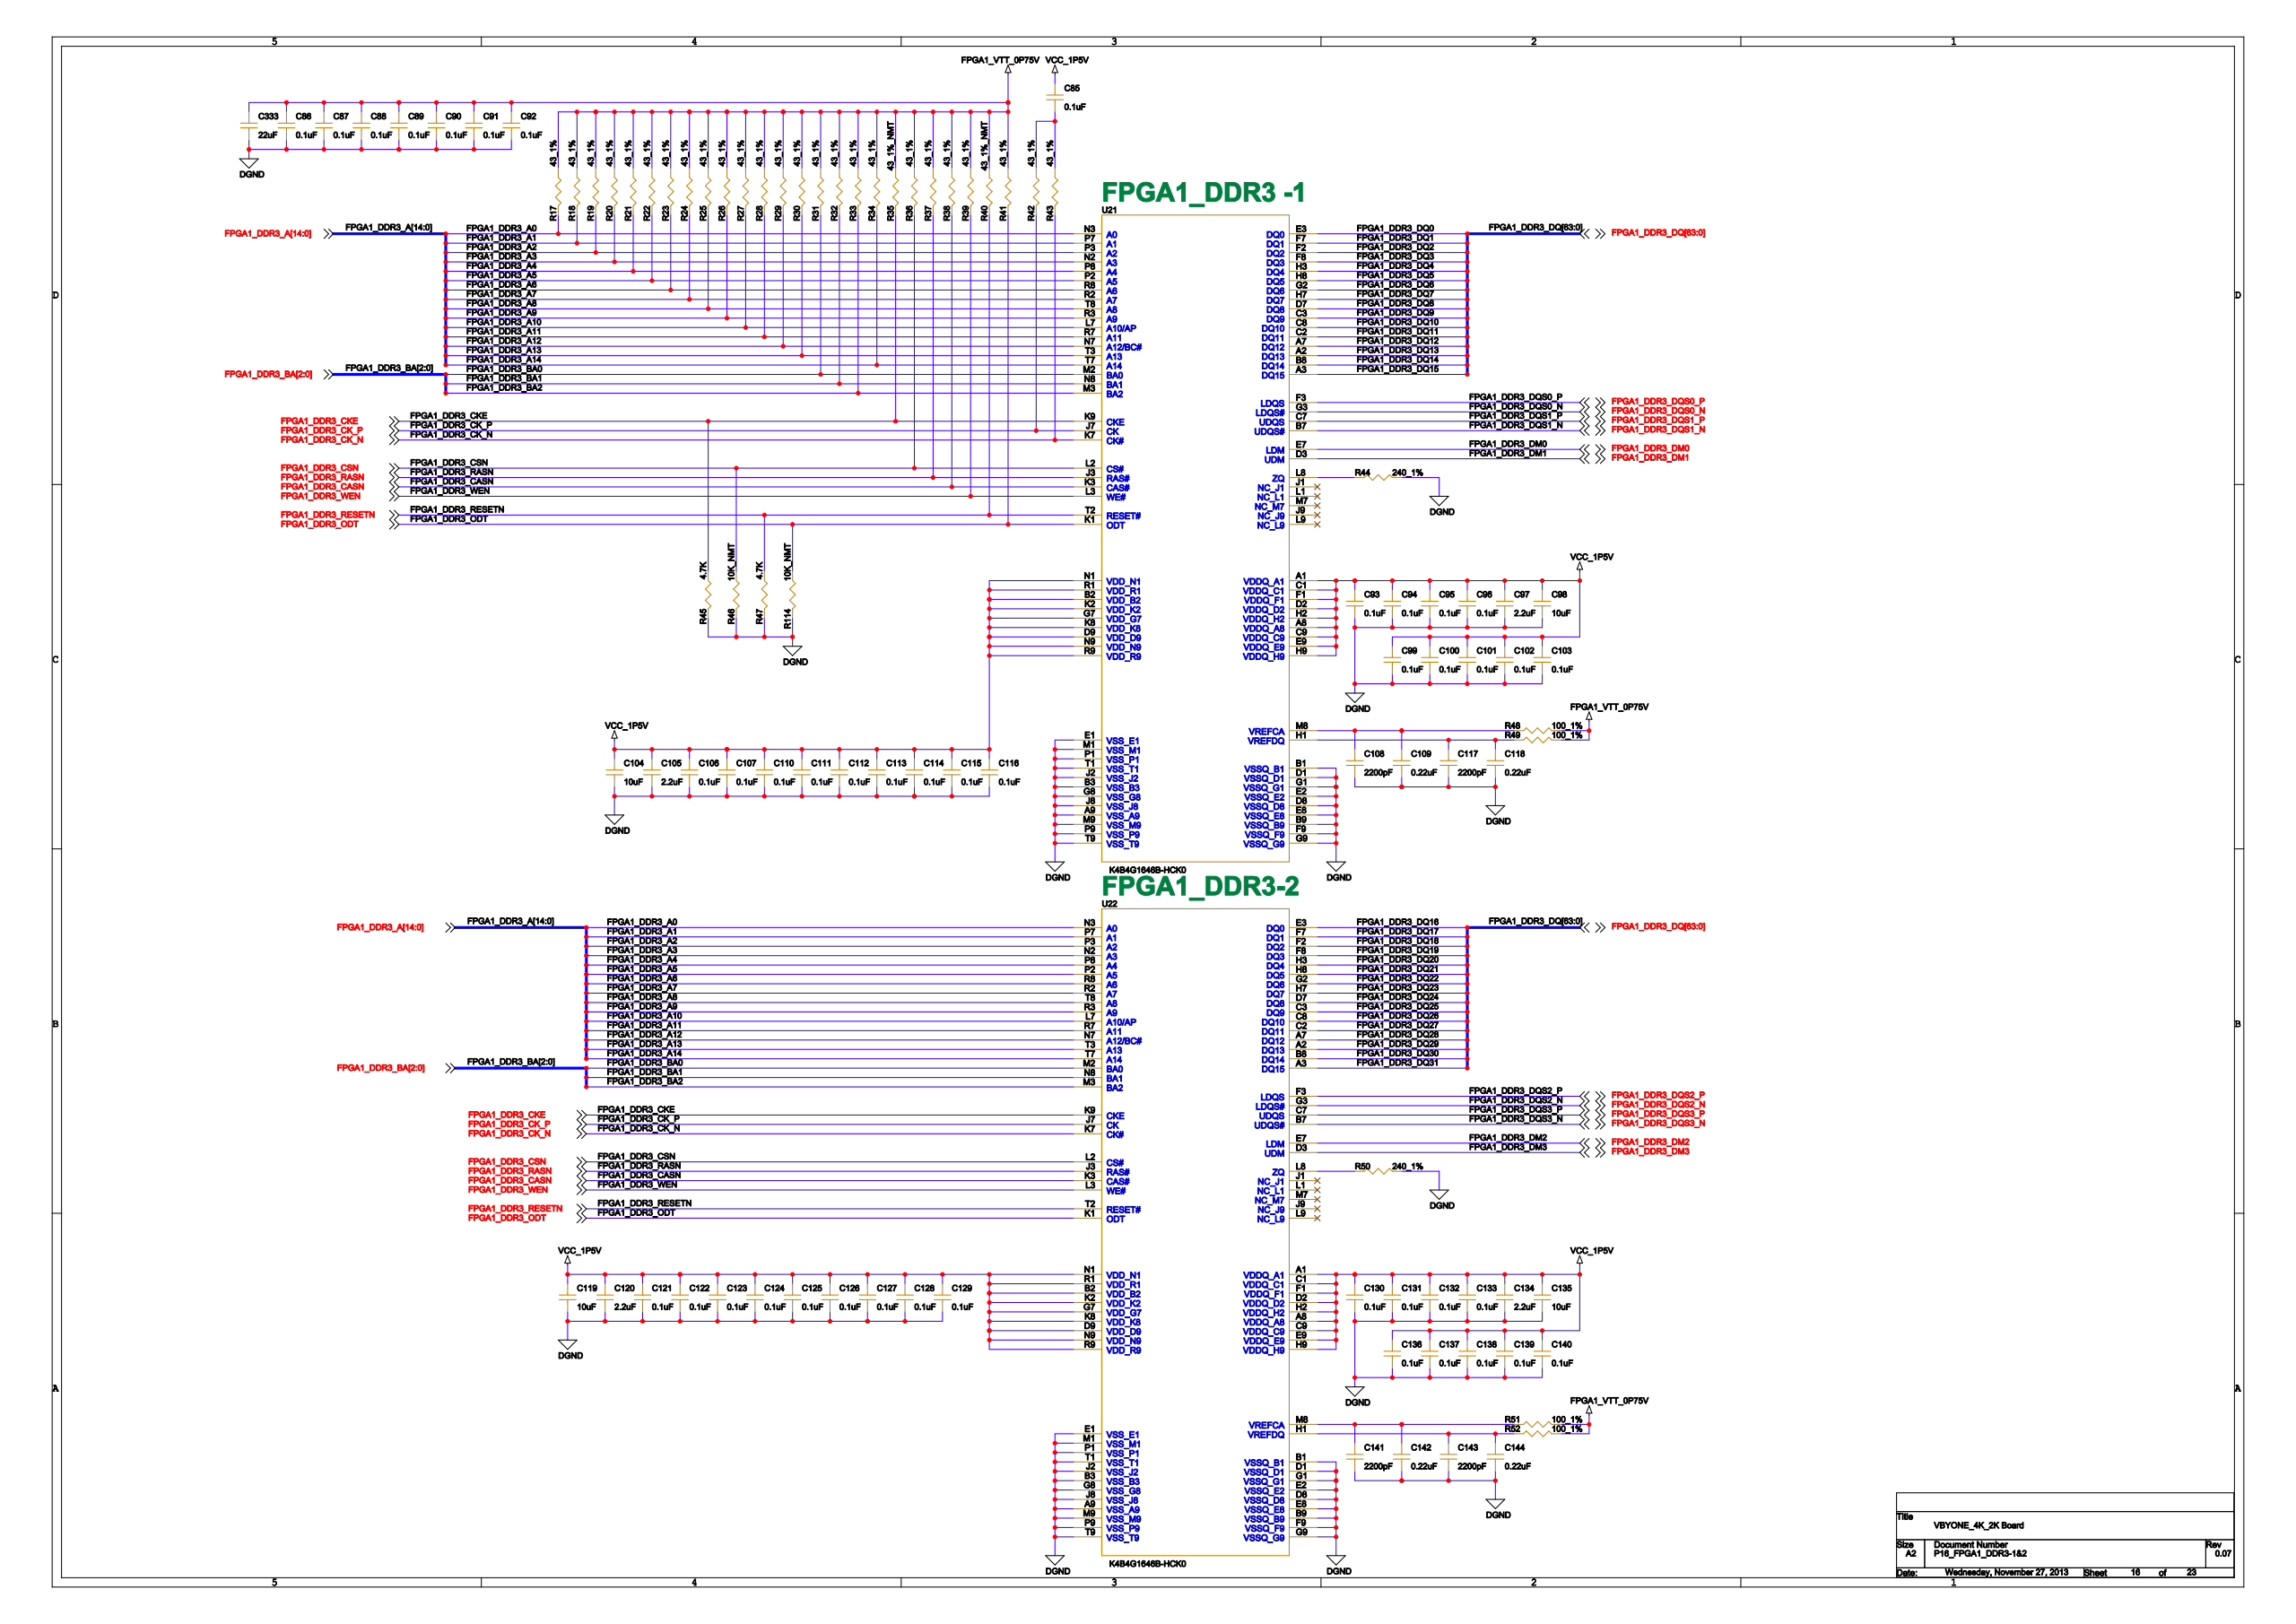Circuit board | Cadence Allegro | 1712 parts | 1495 nets | one sheet of the schematic
Parts on this sheet (reference | value | footprint):
C85 | 0.1uF | CRC1005RZAS
C86 | 0.1uF | CRC1005RZAS
C87 | 0.1uF | CRC1005RZAS
C88 | 0.1uF | CRC1005RZAS
C89 | 0.1uF | CRC1005RZAS
C90 | 0.1uF | CRC1005RZAS
C91 | 0.1uF | CRC1005RZAS
C92 | 0.1uF | CRC1005RZAS
C93 | 0.1uF | CRC1005RZAS
C94 | 0.1uF | CRC1005RZAS
C95 | 0.1uF | CRC1005RZAS
C96 | 0.1uF | CRC1005RZAS
C97 | 2.2uF | CRC1608RZAS
C98 | 10uF | CRC2012RZAS
C99 | 0.1uF | CRC1005RZAS
C100 | 0.1uF | CRC1005RZAS
C101 | 0.1uF | CRC1005RZAS
C102 | 0.1uF | CRC1005RZAS
C103 | 0.1uF | CRC1005RZAS
C104 | 10uF | CRC2012RZAS
C105 | 2.2uF | CRC1608RZAS
C106 | 0.1uF | CRC1005RZAS
C107 | 0.1uF | CRC1005RZAS
C108 | 2200pF | CRC1608RZAS
C109 | 0.22uF | CRC1608RZAS
C110 | 0.1uF | CRC1005RZAS
C111 | 0.1uF | CRC1005RZAS
C112 | 0.1uF | CRC1005RZAS
C113 | 0.1uF | CRC1005RZAS
C114 | 0.1uF | CRC1005RZAS
C115 | 0.1uF | CRC1005RZAS
C116 | 0.1uF | CRC1005RZAS
C117 | 2200pF | CRC1608RZAS
C118 | 0.22uF | CRC1608RZAS
C119 | 10uF | CRC2012RZAS
C120 | 2.2uF | CRC1608RZAS
C121 | 0.1uF | CRC1005RZAS
C122 | 0.1uF | CRC1005RZAS
C123 | 0.1uF | CRC1005RZAS
C124 | 0.1uF | CRC1005RZAS
C125 | 0.1uF | CRC1005RZAS
C126 | 0.1uF | CRC1005RZAS
C127 | 0.1uF | CRC1005RZAS
C128 | 0.1uF | CRC1005RZAS
C129 | 0.1uF | CRC1005RZAS
C130 | 0.1uF | CRC1005RZAS
C131 | 0.1uF | CRC1005RZAS
C132 | 0.1uF | CRC1005RZAS
C133 | 0.1uF | CRC1005RZAS
C134 | 2.2uF | CRC1608RZAS
C135 | 10uF | CRC2012RZAS
C136 | 0.1uF | CRC1005RZAS
C137 | 0.1uF | CRC1005RZAS
C138 | 0.1uF | CRC1005RZAS
C139 | 0.1uF | CRC1005RZAS
C140 | 0.1uF | CRC1005RZAS
C141 | 2200pF | CRC1608RZAS
C142 | 0.22uF | CRC1608RZAS
C143 | 2200pF | CRC1608RZAS
C144 | 0.22uF | CRC1608RZAS
C333 | 22uF | CRC3225RZAS
R17 | 43_1% | CRC1005RZAS
R18 | 43_1% | CRC1005RZAS
R19 | 43_1% | CRC1005RZAS
R20 | 43_1% | CRC1005RZAS
R21 | 43_1% | CRC1005RZAS
R22 | 43_1% | CRC1005RZAS
R23 | 43_1% | CRC1005RZAS
R24 | 43_1% | CRC1005RZAS
R25 | 43_1% | CRC1005RZAS
R26 | 43_1% | CRC1005RZAS
R27 | 43_1% | CRC1005RZAS
R28 | 43_1% | CRC1005RZAS
R29 | 43_1% | CRC1005RZAS
R30 | 43_1% | CRC1005RZAS
R31 | 43_1% | CRC1005RZAS
R32 | 43_1% | CRC1005RZAS
R33 | 43_1% | CRC1005RZAS
R34 | 43_1% | CRC1005RZAS
R35 | 43_1%_NMT | CRC1005RZAS
R36 | 43_1% | CRC1005RZAS
R37 | 43_1% | CRC1005RZAS
R38 | 43_1% | CRC1005RZAS
R39 | 43_1% | CRC1005RZAS
R40 | 43_1%_NMT | CRC1005RZAS
R41 | 43_1% | CRC1005RZAS
R42 | 43_1% | CRC1005RZAS
R43 | 43_1% | CRC1005RZAS
R44 | 240_1% | CRC1608RZAS
R45 | 4.7K | CRC1005RZAS
R46 | 10K_NMT | CRC1005RZAS
R47 | 4.7K | CRC1005RZAS
R48 | 100_1% | CRC1005RZAS
R49 | 100_1% | CRC1005RZAS
R50 | 240_1% | CRC1608RZAS
R51 | 100_1% | CRC1005RZAS
R52 | 100_1% | CRC1005RZAS
R114 | 10K_NMT | CRC1005RZAS
U21 | K4B4G1646B-HCK0 | BGA096RFDS
U22 | K4B4G1646B-HCK0 | BGA096RFDS
Nets of these parts (net: part-pin ...):
DGND: C86-2 C87-2 C88-2 C89-2 C90-2 C91-2 C92-2 C93-2 C94-2 C95-2 C96-2 C97-2 C98-2 C99-2 C100-2 C101-2 C102-2 C103-2 C104-2 C105-2 C106-2 C107-2 C108-2 C109-2 C110-2 C111-2 C112-2 C113-2 C114-2 C115-2 C116-2 C117-2 C118-2 C119-2 C120-2 C121-2 C122-2 C123-2 C124-2 C125-2 C126-2 C127-2 C128-2 C129-2 C130-2 C131-2 C132-2 C133-2 C134-2 C135-2 C136-2 C137-2 C138-2 C139-2 C140-2 C141-2 C142-2 C143-2 C144-2 C333-2 R44-2 R45-2 R46-2 R47-2 R50-2 R114-2 U21-A9 U21-B1 U21-B3 U21-B9 U21-D1 U21-D8 U21-E1 U21-E2 U21-E8 U21-F9 U21-G1 U21-G8 U21-G9 U21-J2 U21-J8 U21-M1 U21-M9 U21-P1 U21-P9 U21-T1 U21-T9 U22-A9 U22-B1 U22-B3 U22-B9 U22-D1 U22-D8 U22-E1 U22-E2 U22-E8 U22-F9 U22-G1 U22-G8 U22-G9 U22-J2 U22-J8 U22-M1 U22-M9 U22-P1 U22-P9 U22-T1 U22-T9
VCC_1P5V: C85-1 C93-1 C94-1 C95-1 C96-1 C97-1 C98-1 C99-1 C100-1 C101-1 C102-1 C103-1 C104-1 C105-1 C106-1 C107-1 C110-1 C111-1 C112-1 C113-1 C114-1 C115-1 C116-1 C119-1 C120-1 C121-1 C122-1 C123-1 C124-1 C125-1 C126-1 C127-1 C128-1 C129-1 C130-1 C131-1 C132-1 C133-1 C134-1 C135-1 C136-1 C137-1 C138-1 C139-1 C140-1 U21-A1 U21-A8 U21-B2 U21-C1 U21-C9 U21-D2 U21-D9 U21-E9 U21-F1 U21-G7 U21-H2 U21-H9 U21-K2 U21-K8 U21-N1 U21-N9 U21-R1 U21-R9 U22-A1 U22-A8 U22-B2 U22-C1 U22-C9 U22-D2 U22-D9 U22-E9 U22-F1 U22-G7 U22-H2 U22-H9 U22-K2 U22-K8 U22-N1 U22-N9 U22-R1 U22-R9
FPGA1_VTT_0P75V: C86-1 C87-1 C88-1 C89-1 C90-1 C91-1 C92-1 C333-1 R17-1 R18-1 R19-1 R20-1 R21-1 R22-1 R23-1 R24-1 R25-1 R26-1 R27-1 R28-1 R29-1 R30-1 R31-1 R32-1 R33-1 R34-1 R35-1 R36-1 R37-1 R38-1 R39-1 R40-1 R41-1 R48-2 R49-2 R51-2 R52-2
N15048264: C85-2 R42-1 R43-1
N15047004: C108-1 C109-1 R48-1 U21-M8
N15047012: C117-1 C118-1 R49-1 U21-H1
N15087599: C141-1 C142-1 R51-1 U22-M8
N15087635: C143-1 C144-1 R52-1 U22-H1
FPGA1_DDR3_CKE: R35-2 R45-1 U21-K9 U22-K9
FPGA1_DDR3_RESETN: R40-2 R47-1 U21-T2 U22-T2
FPGA1_DDR3_ODT: R41-2 R114-1 U21-K1 U22-K1
FPGA1_DDR3_CSN: R36-2 R46-1 U21-L2 U22-L2
FPGA1_DDR3_A0: R17-2 U21-N3 U22-N3
FPGA1_DDR3_A1: R18-2 U21-P7 U22-P7
FPGA1_DDR3_A2: R19-2 U21-P3 U22-P3
FPGA1_DDR3_A3: R20-2 U21-N2 U22-N2
FPGA1_DDR3_A4: R21-2 U21-P8 U22-P8
FPGA1_DDR3_A5: R22-2 U21-P2 U22-P2
FPGA1_DDR3_A6: R23-2 U21-R8 U22-R8
FPGA1_DDR3_A7: R24-2 U21-R2 U22-R2
FPGA1_DDR3_A8: R25-2 U21-T8 U22-T8
FPGA1_DDR3_A9: R26-2 U21-R3 U22-R3
FPGA1_DDR3_A10: R27-2 U21-L7 U22-L7
FPGA1_DDR3_A11: R28-2 U21-R7 U22-R7
FPGA1_DDR3_A12: R29-2 U21-N7 U22-N7
FPGA1_DDR3_A13: R30-2 U21-T3 U22-T3
FPGA1_DDR3_BA0: R31-2 U21-M2 U22-M2
FPGA1_DDR3_BA1: R32-2 U21-N8 U22-N8
FPGA1_DDR3_BA2: R33-2 U21-M3 U22-M3
FPGA1_DDR3_A14: R34-2 U21-T7 U22-T7
FPGA1_DDR3_RASN: R37-2 U21-J3 U22-J3
FPGA1_DDR3_CASN: R38-2 U21-K3 U22-K3
FPGA1_DDR3_WEN: R39-2 U21-L3 U22-L3
FPGA1_DDR3_CK_P: R42-2 U21-J7 U22-J7
FPGA1_DDR3_CK_N: R43-2 U21-K7 U22-K7
N15049798: R44-1 U21-L8
N15089207: R50-1 U22-L8
FPGA1_DDR3_DQ22: U22-G2
FPGA1_DDR3_DQ21: U22-H8
FPGA1_DDR3_DQS2_N: U22-G3
FPGA1_DDR3_DQ10: U21-C8
FPGA1_DDR3_DQ9: U21-C3
FPGA1_DDR3_DQS0_N: U21-G3
FPGA1_DDR3_DQ2: U21-F2
FPGA1_DDR3_DQ20: U22-H3
FPGA1_DDR3_DQ19: U22-F8
FPGA1_DDR3_DQS2_P: U22-F3
FPGA1_DDR3_DQ8: U21-D7
FPGA1_DDR3_DQS0_P: U21-F3
FPGA1_DDR3_DQ1: U21-F7
FPGA1_DDR3_DQ23: U22-H7
FPGA1_DDR3_DQS1_N: U21-B7
FPGA1_DDR3_DM1: U21-D3
FPGA1_DDR3_DQ12: U21-A7
FPGA1_DDR3_DQ0: U21-E3
FPGA1_DDR3_DQ31: U22-A3
FPGA1_DDR3_DQ16: U22-E3
FPGA1_DDR3_DM2: U22-E7
FPGA1_DDR3_DQS1_P: U21-C7
FPGA1_DDR3_DQ11: U21-C2
FPGA1_DDR3_DM0: U21-E7
FPGA1_DDR3_DQ4: U21-H3
FPGA1_DDR3_DQ30: U22-B8
FPGA1_DDR3_DQ18: U22-F2
FPGA1_DDR3_DQ14: U21-B8
FPGA1_DDR3_DQ13: U21-A2
FPGA1_DDR3_DQ3: U21-F8
FPGA1_DDR3_DQ27: U22-C2
FPGA1_DDR3_DQ26: U22-C8
FPGA1_DDR3_DQ17: U22-F7
FPGA1_DDR3_DQ15: U21-A3
FPGA1_DDR3_DQ6: U21-G2
FPGA1_DDR3_DQ5: U21-H8
FPGA1_DDR3_DQS3_N: U22-B7
FPGA1_DDR3_DQS3_P: U22-C7
FPGA1_DDR3_DQ25: U22-C3
FPGA1_DDR3_DQ24: U22-D7
FPGA1_DDR3_DQ7: U21-H7
FPGA1_DDR3_DQ29: U22-A2
FPGA1_DDR3_DQ28: U22-A7
FPGA1_DDR3_DM3: U22-D3